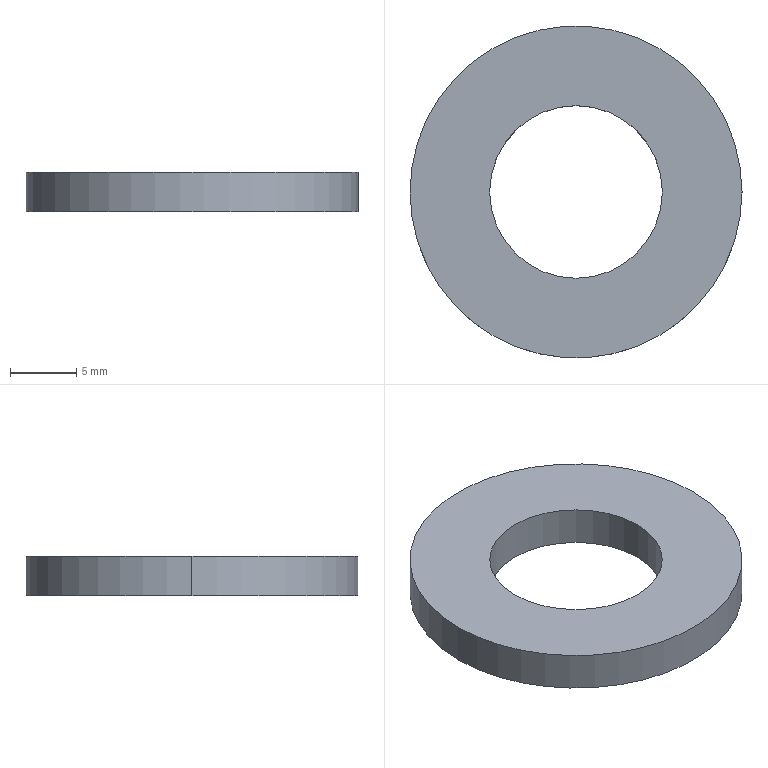Part | SolidWorks | features Extrusion 1 | 1 solid | 6 faces | box 25 x 25 x 3 mm | volume 1074 mm3 | cylinder 4 | plane 2 | commonest cylinder face diameters 13 x2 25 x2
STEP:
#1=CARTESIAN_POINT('',(-6.5,0.,3.));
#2=VERTEX_POINT('',#1);
#3=CARTESIAN_POINT('',(6.5,0.,3.));
#4=VERTEX_POINT('',#3);
#5=CARTESIAN_POINT('',(0.,0.,3.));
#6=DIRECTION('',(0.,0.,1.));
#7=DIRECTION('',(1.,0.,0.));
#8=AXIS2_PLACEMENT_3D('',#5,#6,#7);
#9=CIRCLE('',#8,6.5);
#10=EDGE_CURVE('',#2,#4,#9,.T.);
#11=ORIENTED_EDGE('',*,*,#10,.T.);
#12=CARTESIAN_POINT('',(6.5,0.,0.));
#13=VERTEX_POINT('',#12);
#14=CARTESIAN_POINT('',(6.5,0.,3.));
#15=DIRECTION('',(0.,0.,-1.));
#16=VECTOR('',#15,1000.);
#17=LINE('',#14,#16);
#18=EDGE_CURVE('',#4,#13,#17,.T.);
#19=ORIENTED_EDGE('',*,*,#18,.T.);
#20=CARTESIAN_POINT('',(-6.5,0.,0.));
#21=VERTEX_POINT('',#20);
#22=CARTESIAN_POINT('',(0.,0.,0.));
#23=DIRECTION('',(0.,0.,1.));
#24=DIRECTION('',(1.,0.,0.));
#25=AXIS2_PLACEMENT_3D('',#22,#23,#24);
#26=CIRCLE('',#25,6.5);
#27=EDGE_CURVE('',#21,#13,#26,.T.);
#28=ORIENTED_EDGE('',*,*,#27,.F.);
#29=CARTESIAN_POINT('',(-6.5,0.,3.));
#30=DIRECTION('',(0.,0.,-1.));
#31=VECTOR('',#30,1000.);
#32=LINE('',#29,#31);
#33=EDGE_CURVE('',#2,#21,#32,.T.);
#34=ORIENTED_EDGE('',*,*,#33,.F.);
#35=EDGE_LOOP('',(#11,#19,#28,#34));
#36=FACE_OUTER_BOUND('',#35,.T.);
#37=CARTESIAN_POINT('',(0.,0.,3.));
#38=DIRECTION('',(0.,0.,-1.));
#39=DIRECTION('',(-1.,0.,0.));
#40=AXIS2_PLACEMENT_3D('',#37,#38,#39);
#41=CYLINDRICAL_SURFACE('',#40,6.5);
#42=ADVANCED_FACE('',(#36),#41,.F.);
#43=CARTESIAN_POINT('',(12.5,0.,3.));
#44=VERTEX_POINT('',#43);
#45=CARTESIAN_POINT('',(-12.5,0.,3.));
#46=VERTEX_POINT('',#45);
#47=CARTESIAN_POINT('',(0.,0.,3.));
#48=DIRECTION('',(0.,0.,1.));
#49=DIRECTION('',(1.,0.,0.));
#50=AXIS2_PLACEMENT_3D('',#47,#48,#49);
#51=CIRCLE('',#50,12.5);
#52=EDGE_CURVE('',#44,#46,#51,.T.);
#53=ORIENTED_EDGE('',*,*,#52,.F.);
#54=CARTESIAN_POINT('',(12.5,0.,0.));
#55=VERTEX_POINT('',#54);
#56=CARTESIAN_POINT('',(12.5,0.,3.));
#57=DIRECTION('',(0.,0.,-1.));
#58=VECTOR('',#57,1000.);
#59=LINE('',#56,#58);
#60=EDGE_CURVE('',#44,#55,#59,.T.);
#61=ORIENTED_EDGE('',*,*,#60,.T.);
#62=CARTESIAN_POINT('',(-12.5,0.,0.));
#63=VERTEX_POINT('',#62);
#64=CARTESIAN_POINT('',(0.,0.,0.));
#65=DIRECTION('',(0.,0.,1.));
#66=DIRECTION('',(1.,0.,0.));
#67=AXIS2_PLACEMENT_3D('',#64,#65,#66);
#68=CIRCLE('',#67,12.5);
#69=EDGE_CURVE('',#55,#63,#68,.T.);
#70=ORIENTED_EDGE('',*,*,#69,.T.);
#71=CARTESIAN_POINT('',(-12.5,0.,3.));
#72=DIRECTION('',(0.,0.,-1.));
#73=VECTOR('',#72,1000.);
#74=LINE('',#71,#73);
#75=EDGE_CURVE('',#46,#63,#74,.T.);
#76=ORIENTED_EDGE('',*,*,#75,.F.);
#77=EDGE_LOOP('',(#53,#61,#70,#76));
#78=FACE_OUTER_BOUND('',#77,.T.);
#79=CARTESIAN_POINT('',(0.,0.,3.));
#80=DIRECTION('',(0.,0.,-1.));
#81=DIRECTION('',(-1.,0.,0.));
#82=AXIS2_PLACEMENT_3D('',#79,#80,#81);
#83=CYLINDRICAL_SURFACE('',#82,12.5);
#84=ADVANCED_FACE('',(#78),#83,.T.);
#85=CARTESIAN_POINT('',(0.,0.,3.));
#86=DIRECTION('',(0.,0.,1.));
#87=DIRECTION('',(1.,0.,0.));
#88=AXIS2_PLACEMENT_3D('',#85,#86,#87);
#89=CIRCLE('',#88,12.5);
#90=EDGE_CURVE('',#46,#44,#89,.T.);
#91=ORIENTED_EDGE('',*,*,#90,.T.);
#92=ORIENTED_EDGE('',*,*,#52,.T.);
#93=EDGE_LOOP('',(#91,#92));
#94=FACE_OUTER_BOUND('',#93,.T.);
#95=ORIENTED_EDGE('',*,*,#10,.F.);
#96=CARTESIAN_POINT('',(0.,0.,3.));
#97=DIRECTION('',(0.,0.,1.));
#98=DIRECTION('',(1.,0.,0.));
#99=AXIS2_PLACEMENT_3D('',#96,#97,#98);
#100=CIRCLE('',#99,6.5);
#101=EDGE_CURVE('',#4,#2,#100,.T.);
#102=ORIENTED_EDGE('',*,*,#101,.F.);
#103=EDGE_LOOP('',(#95,#102));
#104=FACE_BOUND('',#103,.T.);
#105=CARTESIAN_POINT('',(0.,0.,3.));
#106=DIRECTION('',(0.,0.,1.));
#107=DIRECTION('',(1.,0.,0.));
#108=AXIS2_PLACEMENT_3D('',#105,#106,#107);
#109=PLANE('',#108);
#110=ADVANCED_FACE('',(#94,#104),#109,.T.);
#111=CARTESIAN_POINT('',(0.,0.,0.));
#112=DIRECTION('',(0.,0.,1.));
#113=DIRECTION('',(1.,0.,0.));
#114=AXIS2_PLACEMENT_3D('',#111,#112,#113);
#115=CIRCLE('',#114,12.5);
#116=EDGE_CURVE('',#63,#55,#115,.T.);
#117=ORIENTED_EDGE('',*,*,#116,.F.);
#118=ORIENTED_EDGE('',*,*,#69,.F.);
#119=EDGE_LOOP('',(#117,#118));
#120=FACE_OUTER_BOUND('',#119,.T.);
#121=ORIENTED_EDGE('',*,*,#27,.T.);
#122=CARTESIAN_POINT('',(0.,0.,0.));
#123=DIRECTION('',(0.,0.,1.));
#124=DIRECTION('',(1.,0.,0.));
#125=AXIS2_PLACEMENT_3D('',#122,#123,#124);
#126=CIRCLE('',#125,6.5);
#127=EDGE_CURVE('',#13,#21,#126,.T.);
#128=ORIENTED_EDGE('',*,*,#127,.T.);
#129=EDGE_LOOP('',(#121,#128));
#130=FACE_BOUND('',#129,.T.);
#131=CARTESIAN_POINT('',(0.,0.,0.));
#132=DIRECTION('',(0.,0.,1.));
#133=DIRECTION('',(1.,0.,0.));
#134=AXIS2_PLACEMENT_3D('',#131,#132,#133);
#135=PLANE('',#134);
#136=ADVANCED_FACE('',(#120,#130),#135,.F.);
#137=ORIENTED_EDGE('',*,*,#60,.F.);
#138=ORIENTED_EDGE('',*,*,#90,.F.);
#139=ORIENTED_EDGE('',*,*,#75,.T.);
#140=ORIENTED_EDGE('',*,*,#116,.T.);
#141=EDGE_LOOP('',(#137,#138,#139,#140));
#142=FACE_OUTER_BOUND('',#141,.T.);
#143=CARTESIAN_POINT('',(0.,0.,3.));
#144=DIRECTION('',(0.,0.,-1.));
#145=DIRECTION('',(-1.,0.,0.));
#146=AXIS2_PLACEMENT_3D('',#143,#144,#145);
#147=CYLINDRICAL_SURFACE('',#146,12.5);
#148=ADVANCED_FACE('',(#142),#147,.T.);
#149=ORIENTED_EDGE('',*,*,#18,.F.);
#150=ORIENTED_EDGE('',*,*,#101,.T.);
#151=ORIENTED_EDGE('',*,*,#33,.T.);
#152=ORIENTED_EDGE('',*,*,#127,.F.);
#153=EDGE_LOOP('',(#149,#150,#151,#152));
#154=FACE_OUTER_BOUND('',#153,.T.);
#155=CARTESIAN_POINT('',(0.,0.,3.));
#156=DIRECTION('',(0.,0.,-1.));
#157=DIRECTION('',(-1.,0.,0.));
#158=AXIS2_PLACEMENT_3D('',#155,#156,#157);
#159=CYLINDRICAL_SURFACE('',#158,6.5);
#160=ADVANCED_FACE('',(#154),#159,.F.);
#161=CLOSED_SHELL('',(#42,#84,#110,#136,#148,#160));
#162=MANIFOLD_SOLID_BREP('',#161);
#163=CARTESIAN_POINT('',(0.,0.,0.));
#164=DIRECTION('',(0.,0.,1.));
#165=DIRECTION('',(1.,0.,0.));
#166=AXIS2_PLACEMENT_3D('',#163,#164,#165);
#167=(LENGTH_UNIT()NAMED_UNIT(*)SI_UNIT(.MILLI.,.METRE.));
#168=UNCERTAINTY_MEASURE_WITH_UNIT(LENGTH_MEASURE(0.00001),#167,'','');
#169=(NAMED_UNIT(*)PLANE_ANGLE_UNIT()SI_UNIT($,.RADIAN.));
#170=(NAMED_UNIT(*)SI_UNIT($,.STERADIAN.)SOLID_ANGLE_UNIT());
#171=(GEOMETRIC_REPRESENTATION_CONTEXT(3)GLOBAL_UNCERTAINTY_ASSIGNED_CONTEXT((#168))GLOBAL_UNIT_ASSIGNED_CONTEXT((#167,#169,#170))REPRESENTATION_CONTEXT('',''));
#172=ADVANCED_BREP_SHAPE_REPRESENTATION('',(#162,#166),#171);